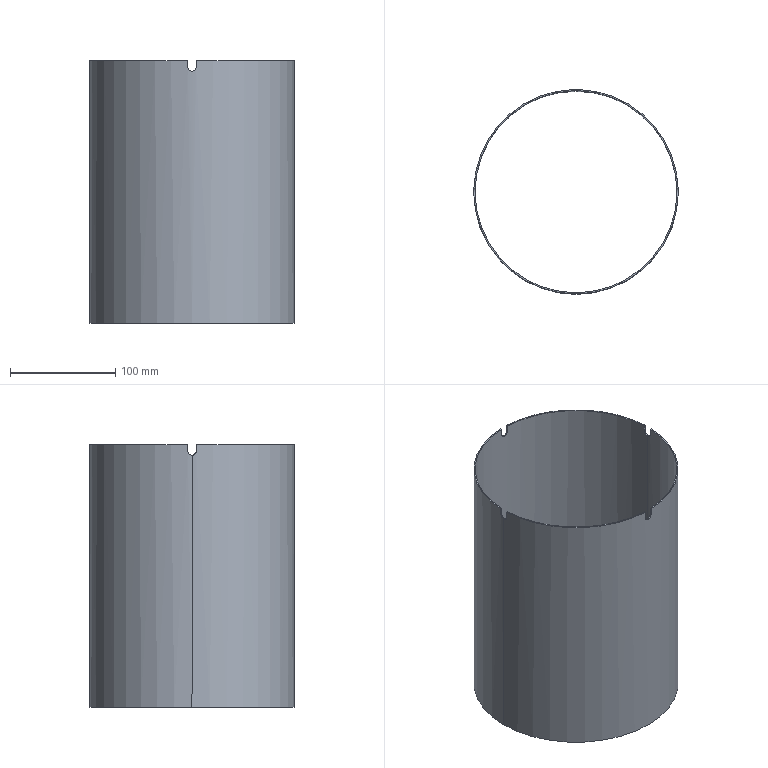Part | SolidWorks | features BaseBody 1 | 1 solid | 23 faces | box 194.5 x 194.5 x 250 mm | volume 181834 mm3 | plane 13 | spline 6 | cylinder 4 | commonest cylinder face diameters 192.1 x2 194.5 x2
STEP:
#1=CARTESIAN_POINT('',(97.25,0.,0.));
#2=VERTEX_POINT('',#1);
#3=CARTESIAN_POINT('',(-97.25,0.,0.));
#4=VERTEX_POINT('',#3);
#5=CARTESIAN_POINT('',(0.,0.,0.));
#6=DIRECTION('',(0.,0.,1.));
#7=DIRECTION('',(1.,0.,0.));
#8=AXIS2_PLACEMENT_3D('',#5,#6,#7);
#9=CIRCLE('',#8,97.25);
#10=EDGE_CURVE('',#2,#4,#9,.T.);
#11=ORIENTED_EDGE('',*,*,#10,.T.);
#12=CARTESIAN_POINT('',(-97.25,0.,240.));
#13=VERTEX_POINT('',#12);
#14=CARTESIAN_POINT('',(-97.25,0.,0.));
#15=DIRECTION('',(0.,0.,1.));
#16=VECTOR('',#15,1000.);
#17=LINE('',#14,#16);
#18=EDGE_CURVE('',#4,#13,#17,.T.);
#19=ORIENTED_EDGE('',*,*,#18,.T.);
#20=CARTESIAN_POINT('',(-97.168,4.,244.));
#21=VERTEX_POINT('',#20);
#22=CARTESIAN_POINT('',(-97.25,0.,240.));
#23=CARTESIAN_POINT('',(-97.25,0.2637,240.002));
#24=CARTESIAN_POINT('',(-97.249,0.5235,240.026));
#25=CARTESIAN_POINT('',(-97.245,1.034,240.127));
#26=CARTESIAN_POINT('',(-97.242,1.287,240.204));
#27=CARTESIAN_POINT('',(-97.234,1.772,240.406));
#28=CARTESIAN_POINT('',(-97.23,2.001,240.528));
#29=CARTESIAN_POINT('',(-97.22,2.437,240.817));
#30=CARTESIAN_POINT('',(-97.214,2.643,240.985));
#31=CARTESIAN_POINT('',(-97.204,3.012,241.354));
#32=CARTESIAN_POINT('',(-97.198,3.177,241.555));
#33=CARTESIAN_POINT('',(-97.188,3.468,241.991));
#34=CARTESIAN_POINT('',(-97.184,3.593,242.225));
#35=CARTESIAN_POINT('',(-97.176,3.794,242.706));
#36=CARTESIAN_POINT('',(-97.173,3.871,242.956));
#37=CARTESIAN_POINT('',(-97.169,3.974,243.474));
#38=CARTESIAN_POINT('',(-97.168,3.999,243.736));
#39=CARTESIAN_POINT('',(-97.168,4.,244.));
#40=B_SPLINE_CURVE_WITH_KNOTS('',3,(#22,#23,#24,#25,#26,#27,#28,#29,#30,#31,#32,#33,#34,#35,#36,#37,#38,#39),.UNSPECIFIED.,.F.,.F.,(4,2,2,2,2,2,2,2,4),(0.,0.0007803,0.001561,0.002341,0.003121,0.003902,0.004682,0.005462,0.006243),.UNSPECIFIED.);
#41=EDGE_CURVE('',#13,#21,#40,.T.);
#42=ORIENTED_EDGE('',*,*,#41,.T.);
#43=CARTESIAN_POINT('',(-97.168,4.,250.));
#44=VERTEX_POINT('',#43);
#45=CARTESIAN_POINT('',(-97.168,4.,0.));
#46=DIRECTION('',(0.,0.,1.));
#47=VECTOR('',#46,1000.);
#48=LINE('',#45,#47);
#49=EDGE_CURVE('',#21,#44,#48,.T.);
#50=ORIENTED_EDGE('',*,*,#49,.T.);
#51=CARTESIAN_POINT('',(-4.,97.168,250.));
#52=VERTEX_POINT('',#51);
#53=CARTESIAN_POINT('',(0.,0.,250.));
#54=DIRECTION('',(0.,0.,-1.));
#55=DIRECTION('',(1.,0.,0.));
#56=AXIS2_PLACEMENT_3D('',#53,#54,#55);
#57=CIRCLE('',#56,97.25);
#58=EDGE_CURVE('',#44,#52,#57,.T.);
#59=ORIENTED_EDGE('',*,*,#58,.T.);
#60=CARTESIAN_POINT('',(-4.,97.168,244.));
#61=VERTEX_POINT('',#60);
#62=CARTESIAN_POINT('',(-4.,97.168,0.));
#63=DIRECTION('',(0.,0.,-1.));
#64=VECTOR('',#63,1000.);
#65=LINE('',#62,#64);
#66=EDGE_CURVE('',#52,#61,#65,.T.);
#67=ORIENTED_EDGE('',*,*,#66,.T.);
#68=CARTESIAN_POINT('',(4.,97.168,244.));
#69=VERTEX_POINT('',#68);
#70=CARTESIAN_POINT('',(-4.,97.168,244.));
#71=CARTESIAN_POINT('',(-3.999,97.168,243.736));
#72=CARTESIAN_POINT('',(-3.974,97.169,243.476));
#73=CARTESIAN_POINT('',(-3.873,97.173,242.965));
#74=CARTESIAN_POINT('',(-3.796,97.176,242.712));
#75=CARTESIAN_POINT('',(-3.594,97.184,242.228));
#76=CARTESIAN_POINT('',(-3.472,97.188,241.998));
#77=CARTESIAN_POINT('',(-3.183,97.198,241.563));
#78=CARTESIAN_POINT('',(-3.014,97.203,241.356));
#79=CARTESIAN_POINT('',(-2.645,97.214,240.987));
#80=CARTESIAN_POINT('',(-2.443,97.22,240.822));
#81=CARTESIAN_POINT('',(-2.007,97.23,240.531));
#82=CARTESIAN_POINT('',(-1.773,97.234,240.406));
#83=CARTESIAN_POINT('',(-1.292,97.242,240.206));
#84=CARTESIAN_POINT('',(-1.041,97.245,240.129));
#85=CARTESIAN_POINT('',(-0.5238,97.249,240.025));
#86=CARTESIAN_POINT('',(-0.2642,97.25,240.));
#87=CARTESIAN_POINT('',(0.2574,97.25,240.));
#88=CARTESIAN_POINT('',(0.5221,97.249,240.026));
#89=CARTESIAN_POINT('',(1.036,97.245,240.128));
#90=CARTESIAN_POINT('',(1.285,97.242,240.203));
#91=CARTESIAN_POINT('',(1.769,97.234,240.403));
#92=CARTESIAN_POINT('',(2.004,97.23,240.528));
#93=CARTESIAN_POINT('',(2.438,97.22,240.818));
#94=CARTESIAN_POINT('',(2.64,97.214,240.983));
#95=CARTESIAN_POINT('',(3.013,97.203,241.355));
#96=CARTESIAN_POINT('',(3.179,97.198,241.558));
#97=CARTESIAN_POINT('',(3.468,97.188,241.992));
#98=CARTESIAN_POINT('',(3.593,97.184,242.225));
#99=CARTESIAN_POINT('',(3.795,97.176,242.71));
#100=CARTESIAN_POINT('',(3.872,97.173,242.959));
#101=CARTESIAN_POINT('',(3.973,97.169,243.471));
#102=CARTESIAN_POINT('',(3.999,97.168,243.736));
#103=CARTESIAN_POINT('',(4.,97.168,244.));
#104=B_SPLINE_CURVE_WITH_KNOTS('',3,(#70,#71,#72,#73,#74,#75,#76,#77,#78,#79,#80,#81,#82,#83,#84,#85,#86,#87,#88,#89,#90,#91,#92,#93,#94,#95,#96,#97,#98,#99,#100,#101,#102,#103),.UNSPECIFIED.,.F.,.F.,(4,2,2,2,2,2,2,2,2,2,2,2,2,2,2,2,4),(0.,0.0007808,0.001562,0.002342,0.003123,0.003904,0.004685,0.005466,0.006246,0.007027,0.007808,0.008589,0.009369,0.01015,0.01093,0.01171,0.01249),.UNSPECIFIED.);
#105=EDGE_CURVE('',#61,#69,#104,.T.);
#106=ORIENTED_EDGE('',*,*,#105,.T.);
#107=CARTESIAN_POINT('',(4.,97.168,250.));
#108=VERTEX_POINT('',#107);
#109=CARTESIAN_POINT('',(4.,97.168,0.));
#110=DIRECTION('',(0.,0.,1.));
#111=VECTOR('',#110,1000.);
#112=LINE('',#109,#111);
#113=EDGE_CURVE('',#69,#108,#112,.T.);
#114=ORIENTED_EDGE('',*,*,#113,.T.);
#115=CARTESIAN_POINT('',(97.168,4.,250.));
#116=VERTEX_POINT('',#115);
#117=CARTESIAN_POINT('',(0.,0.,250.));
#118=DIRECTION('',(0.,0.,-1.));
#119=DIRECTION('',(1.,0.,0.));
#120=AXIS2_PLACEMENT_3D('',#117,#118,#119);
#121=CIRCLE('',#120,97.25);
#122=EDGE_CURVE('',#108,#116,#121,.T.);
#123=ORIENTED_EDGE('',*,*,#122,.T.);
#124=CARTESIAN_POINT('',(97.168,4.,244.));
#125=VERTEX_POINT('',#124);
#126=CARTESIAN_POINT('',(97.168,4.,0.));
#127=DIRECTION('',(0.,0.,-1.));
#128=VECTOR('',#127,1000.);
#129=LINE('',#126,#128);
#130=EDGE_CURVE('',#116,#125,#129,.T.);
#131=ORIENTED_EDGE('',*,*,#130,.T.);
#132=CARTESIAN_POINT('',(97.25,0.,240.));
#133=VERTEX_POINT('',#132);
#134=CARTESIAN_POINT('',(97.168,4.,244.));
#135=CARTESIAN_POINT('',(97.168,3.999,243.736));
#136=CARTESIAN_POINT('',(97.169,3.974,243.476));
#137=CARTESIAN_POINT('',(97.173,3.873,242.966));
#138=CARTESIAN_POINT('',(97.176,3.796,242.713));
#139=CARTESIAN_POINT('',(97.184,3.594,242.228));
#140=CARTESIAN_POINT('',(97.188,3.472,241.999));
#141=CARTESIAN_POINT('',(97.198,3.183,241.563));
#142=CARTESIAN_POINT('',(97.203,3.015,241.357));
#143=CARTESIAN_POINT('',(97.214,2.646,240.988));
#144=CARTESIAN_POINT('',(97.22,2.445,240.823));
#145=CARTESIAN_POINT('',(97.23,2.008,240.532));
#146=CARTESIAN_POINT('',(97.234,1.775,240.407));
#147=CARTESIAN_POINT('',(97.242,1.294,240.206));
#148=CARTESIAN_POINT('',(97.245,1.043,240.129));
#149=CARTESIAN_POINT('',(97.249,0.5258,240.026));
#150=CARTESIAN_POINT('',(97.25,0.2641,240.002));
#151=CARTESIAN_POINT('',(97.25,0.,240.));
#152=B_SPLINE_CURVE_WITH_KNOTS('',3,(#134,#135,#136,#137,#138,#139,#140,#141,#142,#143,#144,#145,#146,#147,#148,#149,#150,#151),.UNSPECIFIED.,.F.,.F.,(4,2,2,2,2,2,2,2,4),(0.,0.0007804,0.001561,0.002341,0.003122,0.003902,0.004683,0.005463,0.006243),.UNSPECIFIED.);
#153=EDGE_CURVE('',#125,#133,#152,.T.);
#154=ORIENTED_EDGE('',*,*,#153,.T.);
#155=CARTESIAN_POINT('',(97.25,0.,0.));
#156=DIRECTION('',(0.,0.,1.));
#157=VECTOR('',#156,1000.);
#158=LINE('',#155,#157);
#159=EDGE_CURVE('',#2,#133,#158,.T.);
#160=ORIENTED_EDGE('',*,*,#159,.F.);
#161=EDGE_LOOP('',(#11,#19,#42,#50,#59,#67,#106,#114,#123,#131,#154,#160));
#162=FACE_OUTER_BOUND('',#161,.T.);
#163=CARTESIAN_POINT('',(0.,0.,0.));
#164=DIRECTION('',(0.,0.,1.));
#165=DIRECTION('',(1.,0.,0.));
#166=AXIS2_PLACEMENT_3D('',#163,#164,#165);
#167=CYLINDRICAL_SURFACE('',#166,97.25);
#168=ADVANCED_FACE('',(#162),#167,.T.);
#169=CARTESIAN_POINT('',(-96.05,0.,0.));
#170=VERTEX_POINT('',#169);
#171=CARTESIAN_POINT('',(96.05,0.,0.));
#172=VERTEX_POINT('',#171);
#173=CARTESIAN_POINT('',(0.,0.,0.));
#174=DIRECTION('',(0.,0.,1.));
#175=DIRECTION('',(1.,0.,0.));
#176=AXIS2_PLACEMENT_3D('',#173,#174,#175);
#177=CIRCLE('',#176,96.05);
#178=EDGE_CURVE('',#170,#172,#177,.T.);
#179=ORIENTED_EDGE('',*,*,#178,.F.);
#180=CARTESIAN_POINT('',(-96.05,0.,240.));
#181=VERTEX_POINT('',#180);
#182=CARTESIAN_POINT('',(-96.05,0.,0.));
#183=DIRECTION('',(0.,0.,1.));
#184=VECTOR('',#183,1000.);
#185=LINE('',#182,#184);
#186=EDGE_CURVE('',#170,#181,#185,.T.);
#187=ORIENTED_EDGE('',*,*,#186,.T.);
#188=CARTESIAN_POINT('',(-95.969,-3.951,244.));
#189=VERTEX_POINT('',#188);
#190=CARTESIAN_POINT('',(-96.05,0.,240.));
#191=CARTESIAN_POINT('',(-96.05,-0.2623,240.001));
#192=CARTESIAN_POINT('',(-96.049,-0.5205,240.026));
#193=CARTESIAN_POINT('',(-96.045,-1.028,240.129));
#194=CARTESIAN_POINT('',(-96.042,-1.28,240.207));
#195=CARTESIAN_POINT('',(-96.034,-1.759,240.41));
#196=CARTESIAN_POINT('',(-96.03,-1.987,240.533));
#197=CARTESIAN_POINT('',(-96.02,-2.417,240.824));
#198=CARTESIAN_POINT('',(-96.014,-2.62,240.994));
#199=CARTESIAN_POINT('',(-96.004,-2.982,241.364));
#200=CARTESIAN_POINT('',(-95.999,-3.145,241.566));
#201=CARTESIAN_POINT('',(-95.989,-3.433,242.003));
#202=CARTESIAN_POINT('',(-95.984,-3.554,242.235));
#203=CARTESIAN_POINT('',(-95.977,-3.749,242.714));
#204=CARTESIAN_POINT('',(-95.974,-3.825,242.965));
#205=CARTESIAN_POINT('',(-95.97,-3.926,243.478));
#206=CARTESIAN_POINT('',(-95.969,-3.95,243.738));
#207=CARTESIAN_POINT('',(-95.969,-3.951,244.));
#208=B_SPLINE_CURVE_WITH_KNOTS('',3,(#190,#191,#192,#193,#194,#195,#196,#197,#198,#199,#200,#201,#202,#203,#204,#205,#206,#207),.UNSPECIFIED.,.F.,.F.,(4,2,2,2,2,2,2,2,4),(0.,0.000776,0.001552,0.002328,0.003104,0.00388,0.004656,0.005432,0.006208),.UNSPECIFIED.);
#209=EDGE_CURVE('',#181,#189,#208,.T.);
#210=ORIENTED_EDGE('',*,*,#209,.T.);
#211=CARTESIAN_POINT('',(-95.969,-3.951,250.));
#212=VERTEX_POINT('',#211);
#213=CARTESIAN_POINT('',(-95.969,-3.951,247.));
#214=DIRECTION('',(0.,0.,1.));
#215=VECTOR('',#214,1000.);
#216=LINE('',#213,#215);
#217=EDGE_CURVE('',#189,#212,#216,.T.);
#218=ORIENTED_EDGE('',*,*,#217,.T.);
#219=CARTESIAN_POINT('',(-3.951,-95.969,250.));
#220=VERTEX_POINT('',#219);
#221=CARTESIAN_POINT('',(0.,0.,250.));
#222=DIRECTION('',(0.,0.,1.));
#223=DIRECTION('',(1.,0.,0.));
#224=AXIS2_PLACEMENT_3D('',#221,#222,#223);
#225=CIRCLE('',#224,96.05);
#226=EDGE_CURVE('',#212,#220,#225,.T.);
#227=ORIENTED_EDGE('',*,*,#226,.T.);
#228=CARTESIAN_POINT('',(-3.951,-95.969,244.));
#229=VERTEX_POINT('',#228);
#230=CARTESIAN_POINT('',(-3.951,-95.969,247.));
#231=DIRECTION('',(0.,0.,1.));
#232=VECTOR('',#231,1000.);
#233=LINE('',#230,#232);
#234=EDGE_CURVE('',#229,#220,#233,.T.);
#235=ORIENTED_EDGE('',*,*,#234,.F.);
#236=CARTESIAN_POINT('',(3.951,-95.969,244.));
#237=VERTEX_POINT('',#236);
#238=CARTESIAN_POINT('',(-3.951,-95.969,244.));
#239=CARTESIAN_POINT('',(-3.949,-95.969,243.738));
#240=CARTESIAN_POINT('',(-3.925,-95.97,243.479));
#241=CARTESIAN_POINT('',(-3.827,-95.974,242.972));
#242=CARTESIAN_POINT('',(-3.751,-95.977,242.72));
#243=CARTESIAN_POINT('',(-3.554,-95.984,242.237));
#244=CARTESIAN_POINT('',(-3.434,-95.989,242.007));
#245=CARTESIAN_POINT('',(-3.151,-95.998,241.573));
#246=CARTESIAN_POINT('',(-2.985,-96.004,241.366));
#247=CARTESIAN_POINT('',(-2.622,-96.014,240.996));
#248=CARTESIAN_POINT('',(-2.423,-96.02,240.83));
#249=CARTESIAN_POINT('',(-1.993,-96.03,240.537));
#250=CARTESIAN_POINT('',(-1.761,-96.034,240.41));
#251=CARTESIAN_POINT('',(-1.284,-96.042,240.208));
#252=CARTESIAN_POINT('',(-1.036,-96.045,240.131));
#253=CARTESIAN_POINT('',(-0.5214,-96.049,240.026));
#254=CARTESIAN_POINT('',(-0.2631,-96.05,240.));
#255=CARTESIAN_POINT('',(0.255,-96.05,240.));
#256=CARTESIAN_POINT('',(0.5178,-96.049,240.026));
#257=CARTESIAN_POINT('',(1.029,-96.045,240.129));
#258=CARTESIAN_POINT('',(1.276,-96.042,240.205));
#259=CARTESIAN_POINT('',(1.756,-96.034,240.407));
#260=CARTESIAN_POINT('',(1.988,-96.03,240.534));
#261=CARTESIAN_POINT('',(2.417,-96.02,240.825));
#262=CARTESIAN_POINT('',(2.616,-96.015,240.991));
#263=CARTESIAN_POINT('',(2.984,-96.004,241.365));
#264=CARTESIAN_POINT('',(3.147,-95.999,241.568));
#265=CARTESIAN_POINT('',(3.431,-95.989,242.001));
#266=CARTESIAN_POINT('',(3.553,-95.984,242.234));
#267=CARTESIAN_POINT('',(3.751,-95.977,242.717));
#268=CARTESIAN_POINT('',(3.825,-95.974,242.965));
#269=CARTESIAN_POINT('',(3.925,-95.97,243.475));
#270=CARTESIAN_POINT('',(3.949,-95.969,243.737));
#271=CARTESIAN_POINT('',(3.951,-95.969,244.));
#272=B_SPLINE_CURVE_WITH_KNOTS('',3,(#238,#239,#240,#241,#242,#243,#244,#245,#246,#247,#248,#249,#250,#251,#252,#253,#254,#255,#256,#257,#258,#259,#260,#261,#262,#263,#264,#265,#266,#267,#268,#269,#270,#271),.UNSPECIFIED.,.F.,.F.,(4,2,2,2,2,2,2,2,2,2,2,2,2,2,2,2,4),(0.,0.0007758,0.001552,0.002328,0.003103,0.003879,0.004655,0.005431,0.006207,0.006983,0.007758,0.008534,0.00931,0.01009,0.01086,0.01164,0.01241),.UNSPECIFIED.);
#273=EDGE_CURVE('',#229,#237,#272,.T.);
#274=ORIENTED_EDGE('',*,*,#273,.T.);
#275=CARTESIAN_POINT('',(3.951,-95.969,250.));
#276=VERTEX_POINT('',#275);
#277=CARTESIAN_POINT('',(3.951,-95.969,247.));
#278=DIRECTION('',(0.,0.,1.));
#279=VECTOR('',#278,1000.);
#280=LINE('',#277,#279);
#281=EDGE_CURVE('',#237,#276,#280,.T.);
#282=ORIENTED_EDGE('',*,*,#281,.T.);
#283=CARTESIAN_POINT('',(95.969,-3.951,250.));
#284=VERTEX_POINT('',#283);
#285=CARTESIAN_POINT('',(0.,0.,250.));
#286=DIRECTION('',(0.,0.,1.));
#287=DIRECTION('',(1.,0.,0.));
#288=AXIS2_PLACEMENT_3D('',#285,#286,#287);
#289=CIRCLE('',#288,96.05);
#290=EDGE_CURVE('',#276,#284,#289,.T.);
#291=ORIENTED_EDGE('',*,*,#290,.T.);
#292=CARTESIAN_POINT('',(95.969,-3.951,244.));
#293=VERTEX_POINT('',#292);
#294=CARTESIAN_POINT('',(95.969,-3.951,247.));
#295=DIRECTION('',(0.,0.,1.));
#296=VECTOR('',#295,1000.);
#297=LINE('',#294,#296);
#298=EDGE_CURVE('',#293,#284,#297,.T.);
#299=ORIENTED_EDGE('',*,*,#298,.F.);
#300=CARTESIAN_POINT('',(96.05,0.,240.));
#301=VERTEX_POINT('',#300);
#302=CARTESIAN_POINT('',(95.969,-3.951,244.));
#303=CARTESIAN_POINT('',(95.969,-3.95,243.738));
#304=CARTESIAN_POINT('',(95.97,-3.926,243.479));
#305=CARTESIAN_POINT('',(95.974,-3.826,242.972));
#306=CARTESIAN_POINT('',(95.977,-3.751,242.719));
#307=CARTESIAN_POINT('',(95.984,-3.555,242.236));
#308=CARTESIAN_POINT('',(95.989,-3.435,242.007));
#309=CARTESIAN_POINT('',(95.998,-3.151,241.574));
#310=CARTESIAN_POINT('',(96.004,-2.985,241.367));
#311=CARTESIAN_POINT('',(96.014,-2.622,240.996));
#312=CARTESIAN_POINT('',(96.02,-2.424,240.83));
#313=CARTESIAN_POINT('',(96.03,-1.994,240.537));
#314=CARTESIAN_POINT('',(96.034,-1.762,240.411));
#315=CARTESIAN_POINT('',(96.042,-1.285,240.209));
#316=CARTESIAN_POINT('',(96.045,-1.037,240.131));
#317=CARTESIAN_POINT('',(96.049,-0.5226,240.026));
#318=CARTESIAN_POINT('',(96.05,-0.2626,240.));
#319=CARTESIAN_POINT('',(96.05,0.,240.));
#320=B_SPLINE_CURVE_WITH_KNOTS('',3,(#302,#303,#304,#305,#306,#307,#308,#309,#310,#311,#312,#313,#314,#315,#316,#317,#318,#319),.UNSPECIFIED.,.F.,.F.,(4,2,2,2,2,2,2,2,4),(0.,0.000776,0.001552,0.002328,0.003104,0.00388,0.004656,0.005432,0.006208),.UNSPECIFIED.);
#321=EDGE_CURVE('',#293,#301,#320,.T.);
#322=ORIENTED_EDGE('',*,*,#321,.T.);
#323=CARTESIAN_POINT('',(96.05,0.,0.));
#324=DIRECTION('',(0.,0.,1.));
#325=VECTOR('',#324,1000.);
#326=LINE('',#323,#325);
#327=EDGE_CURVE('',#172,#301,#326,.T.);
#328=ORIENTED_EDGE('',*,*,#327,.F.);
#329=EDGE_LOOP('',(#179,#187,#210,#218,#227,#235,#274,#282,#291,#299,#322,#328));
#330=FACE_OUTER_BOUND('',#329,.T.);
#331=CARTESIAN_POINT('',(0.,0.,0.));
#332=DIRECTION('',(0.,0.,1.));
#333=DIRECTION('',(1.,0.,0.));
#334=AXIS2_PLACEMENT_3D('',#331,#332,#333);
#335=CYLINDRICAL_SURFACE('',#334,96.05);
#336=ADVANCED_FACE('',(#330),#335,.F.);
#337=ORIENTED_EDGE('',*,*,#18,.F.);
#338=CARTESIAN_POINT('',(0.,0.,0.));
#339=DIRECTION('',(0.,0.,1.));
#340=DIRECTION('',(1.,0.,0.));
#341=AXIS2_PLACEMENT_3D('',#338,#339,#340);
#342=CIRCLE('',#341,97.25);
#343=EDGE_CURVE('',#4,#2,#342,.T.);
#344=ORIENTED_EDGE('',*,*,#343,.T.);
#345=ORIENTED_EDGE('',*,*,#159,.T.);
#346=CARTESIAN_POINT('',(97.168,-4.,244.));
#347=VERTEX_POINT('',#346);
#348=CARTESIAN_POINT('',(97.25,0.,240.));
#349=CARTESIAN_POINT('',(97.25,-0.2639,240.));
#350=CARTESIAN_POINT('',(97.249,-0.5237,240.025));
#351=CARTESIAN_POINT('',(97.245,-1.034,240.127));
#352=CARTESIAN_POINT('',(97.242,-1.288,240.205));
#353=CARTESIAN_POINT('',(97.234,-1.772,240.405));
#354=CARTESIAN_POINT('',(97.23,-2.002,240.527));
#355=CARTESIAN_POINT('',(97.22,-2.437,240.817));
#356=CARTESIAN_POINT('',(97.214,-2.643,240.986));
#357=CARTESIAN_POINT('',(97.204,-3.012,241.355));
#358=CARTESIAN_POINT('',(97.198,-3.177,241.556));
#359=CARTESIAN_POINT('',(97.188,-3.47,241.993));
#360=CARTESIAN_POINT('',(97.184,-3.594,242.226));
#361=CARTESIAN_POINT('',(97.176,-3.794,242.706));
#362=CARTESIAN_POINT('',(97.173,-3.871,242.958));
#363=CARTESIAN_POINT('',(97.169,-3.974,243.475));
#364=CARTESIAN_POINT('',(97.168,-3.999,243.736));
#365=CARTESIAN_POINT('',(97.168,-4.,244.));
#366=B_SPLINE_CURVE_WITH_KNOTS('',3,(#348,#349,#350,#351,#352,#353,#354,#355,#356,#357,#358,#359,#360,#361,#362,#363,#364,#365),.UNSPECIFIED.,.F.,.F.,(4,2,2,2,2,2,2,2,4),(0.,0.0007808,0.001562,0.002342,0.003123,0.003904,0.004685,0.005466,0.006247),.UNSPECIFIED.);
#367=EDGE_CURVE('',#133,#347,#366,.T.);
#368=ORIENTED_EDGE('',*,*,#367,.T.);
#369=CARTESIAN_POINT('',(97.168,-4.,250.));
#370=VERTEX_POINT('',#369);
#371=CARTESIAN_POINT('',(97.168,-4.,0.));
#372=DIRECTION('',(0.,0.,1.));
#373=VECTOR('',#372,1000.);
#374=LINE('',#371,#373);
#375=EDGE_CURVE('',#347,#370,#374,.T.);
#376=ORIENTED_EDGE('',*,*,#375,.T.);
#377=CARTESIAN_POINT('',(4.,-97.168,250.));
#378=VERTEX_POINT('',#377);
#379=CARTESIAN_POINT('',(0.,0.,250.));
#380=DIRECTION('',(0.,0.,-1.));
#381=DIRECTION('',(1.,0.,0.));
#382=AXIS2_PLACEMENT_3D('',#379,#380,#381);
#383=CIRCLE('',#382,97.25);
#384=EDGE_CURVE('',#370,#378,#383,.T.);
#385=ORIENTED_EDGE('',*,*,#384,.T.);
#386=CARTESIAN_POINT('',(4.,-97.168,244.));
#387=VERTEX_POINT('',#386);
#388=CARTESIAN_POINT('',(4.,-97.168,0.));
#389=DIRECTION('',(0.,0.,-1.));
#390=VECTOR('',#389,1000.);
#391=LINE('',#388,#390);
#392=EDGE_CURVE('',#378,#387,#391,.T.);
#393=ORIENTED_EDGE('',*,*,#392,.T.);
#394=CARTESIAN_POINT('',(-4.,-97.168,244.));
#395=VERTEX_POINT('',#394);
#396=CARTESIAN_POINT('',(4.,-97.168,244.));
#397=CARTESIAN_POINT('',(3.999,-97.168,243.736));
#398=CARTESIAN_POINT('',(3.974,-97.169,243.476));
#399=CARTESIAN_POINT('',(3.873,-97.173,242.965));
#400=CARTESIAN_POINT('',(3.796,-97.176,242.712));
#401=CARTESIAN_POINT('',(3.594,-97.184,242.228));
#402=CARTESIAN_POINT('',(3.472,-97.188,241.998));
#403=CARTESIAN_POINT('',(3.183,-97.198,241.563));
#404=CARTESIAN_POINT('',(3.014,-97.203,241.357));
#405=CARTESIAN_POINT('',(2.645,-97.214,240.988));
#406=CARTESIAN_POINT('',(2.443,-97.22,240.822));
#407=CARTESIAN_POINT('',(2.007,-97.23,240.53));
#408=CARTESIAN_POINT('',(1.774,-97.234,240.405));
#409=CARTESIAN_POINT('',(1.292,-97.242,240.205));
#410=CARTESIAN_POINT('',(1.041,-97.245,240.129));
#411=CARTESIAN_POINT('',(0.5239,-97.249,240.026));
#412=CARTESIAN_POINT('',(0.2642,-97.25,240.));
#413=CARTESIAN_POINT('',(-0.2575,-97.25,240.));
#414=CARTESIAN_POINT('',(-0.5223,-97.249,240.025));
#415=CARTESIAN_POINT('',(-1.036,-97.245,240.127));
#416=CARTESIAN_POINT('',(-1.285,-97.242,240.203));
#417=CARTESIAN_POINT('',(-1.769,-97.234,240.404));
#418=CARTESIAN_POINT('',(-2.003,-97.23,240.529));
#419=CARTESIAN_POINT('',(-2.438,-97.22,240.818));
#420=CARTESIAN_POINT('',(-2.64,-97.214,240.983));
#421=CARTESIAN_POINT('',(-3.013,-97.203,241.355));
#422=CARTESIAN_POINT('',(-3.179,-97.198,241.558));
#423=CARTESIAN_POINT('',(-3.468,-97.188,241.992));
#424=CARTESIAN_POINT('',(-3.593,-97.184,242.225));
#425=CARTESIAN_POINT('',(-3.795,-97.176,242.71));
#426=CARTESIAN_POINT('',(-3.872,-97.173,242.959));
#427=CARTESIAN_POINT('',(-3.973,-97.169,243.471));
#428=CARTESIAN_POINT('',(-3.999,-97.168,243.736));
#429=CARTESIAN_POINT('',(-4.,-97.168,244.));
#430=B_SPLINE_CURVE_WITH_KNOTS('',3,(#396,#397,#398,#399,#400,#401,#402,#403,#404,#405,#406,#407,#408,#409,#410,#411,#412,#413,#414,#415,#416,#417,#418,#419,#420,#421,#422,#423,#424,#425,#426,#427,#428,#429),.UNSPECIFIED.,.F.,.F.,(4,2,2,2,2,2,2,2,2,2,2,2,2,2,2,2,4),(0.,0.0007808,0.001562,0.002342,0.003123,0.003904,0.004685,0.005466,0.006246,0.007027,0.007808,0.008589,0.009369,0.01015,0.01093,0.01171,0.01249),.UNSPECIFIED.);
#431=EDGE_CURVE('',#387,#395,#430,.T.);
#432=ORIENTED_EDGE('',*,*,#431,.T.);
#433=CARTESIAN_POINT('',(-4.,-97.168,250.));
#434=VERTEX_POINT('',#433);
#435=CARTESIAN_POINT('',(-4.,-97.168,0.));
#436=DIRECTION('',(0.,0.,1.));
#437=VECTOR('',#436,1000.);
#438=LINE('',#435,#437);
#439=EDGE_CURVE('',#395,#434,#438,.T.);
#440=ORIENTED_EDGE('',*,*,#439,.T.);
#441=CARTESIAN_POINT('',(-97.168,-4.,250.));
#442=VERTEX_POINT('',#441);
#443=CARTESIAN_POINT('',(0.,0.,250.));
#444=DIRECTION('',(0.,0.,-1.));
#445=DIRECTION('',(1.,0.,0.));
#446=AXIS2_PLACEMENT_3D('',#443,#444,#445);
#447=CIRCLE('',#446,97.25);
#448=EDGE_CURVE('',#434,#442,#447,.T.);
#449=ORIENTED_EDGE('',*,*,#448,.T.);
#450=CARTESIAN_POINT('',(-97.168,-4.,244.));
#451=VERTEX_POINT('',#450);
#452=CARTESIAN_POINT('',(-97.168,-4.,0.));
#453=DIRECTION('',(0.,0.,-1.));
#454=VECTOR('',#453,1000.);
#455=LINE('',#452,#454);
#456=EDGE_CURVE('',#442,#451,#455,.T.);
#457=ORIENTED_EDGE('',*,*,#456,.T.);
#458=CARTESIAN_POINT('',(-97.168,-4.,244.));
#459=CARTESIAN_POINT('',(-97.168,-3.999,243.736));
#460=CARTESIAN_POINT('',(-97.169,-3.974,243.476));
#461=CARTESIAN_POINT('',(-97.173,-3.873,242.965));
#462=CARTESIAN_POINT('',(-97.176,-3.796,242.712));
#463=CARTESIAN_POINT('',(-97.184,-3.595,242.228));
#464=CARTESIAN_POINT('',(-97.188,-3.473,241.998));
#465=CARTESIAN_POINT('',(-97.198,-3.183,241.564));
#466=CARTESIAN_POINT('',(-97.203,-3.014,241.358));
#467=CARTESIAN_POINT('',(-97.214,-2.646,240.988));
#468=CARTESIAN_POINT('',(-97.22,-2.445,240.822));
#469=CARTESIAN_POINT('',(-97.23,-2.008,240.531));
#470=CARTESIAN_POINT('',(-97.234,-1.775,240.407));
#471=CARTESIAN_POINT('',(-97.242,-1.294,240.207));
#472=CARTESIAN_POINT('',(-97.245,-1.043,240.129));
#473=CARTESIAN_POINT('',(-97.249,-0.5256,240.025));
#474=CARTESIAN_POINT('',(-97.25,-0.2641,240.001));
#475=CARTESIAN_POINT('',(-97.25,0.,240.));
#476=B_SPLINE_CURVE_WITH_KNOTS('',3,(#458,#459,#460,#461,#462,#463,#464,#465,#466,#467,#468,#469,#470,#471,#472,#473,#474,#475),.UNSPECIFIED.,.F.,.F.,(4,2,2,2,2,2,2,2,4),(0.,0.0007809,0.001562,0.002343,0.003123,0.003904,0.004685,0.005466,0.006247),.UNSPECIFIED.);
#477=EDGE_CURVE('',#451,#13,#476,.T.);
#478=ORIENTED_EDGE('',*,*,#477,.T.);
#479=EDGE_LOOP('',(#337,#344,#345,#368,#376,#385,#393,#432,#440,#449,#457,#478));
#480=FACE_OUTER_BOUND('',#479,.T.);
#481=CARTESIAN_POINT('',(0.,0.,0.));
#482=DIRECTION('',(0.,0.,1.));
#483=DIRECTION('',(1.,0.,0.));
#484=AXIS2_PLACEMENT_3D('',#481,#482,#483);
#485=CYLINDRICAL_SURFACE('',#484,97.25);
#486=ADVANCED_FACE('',(#480),#485,.T.);
#487=CARTESIAN_POINT('',(3.951,95.969,250.));
#488=VERTEX_POINT('',#487);
#489=CARTESIAN_POINT('',(3.975,96.568,250.));
#490=DIRECTION('',(0.04113,0.9992,0.));
#491=VECTOR('',#490,1000.);
#492=LINE('',#489,#491);
#493=EDGE_CURVE('',#488,#108,#492,.T.);
#494=ORIENTED_EDGE('',*,*,#493,.T.);
#495=ORIENTED_EDGE('',*,*,#113,.F.);
#496=CARTESIAN_POINT('',(3.951,95.969,244.));
#497=VERTEX_POINT('',#496);
#498=CARTESIAN_POINT('',(3.975,96.568,244.));
#499=DIRECTION('',(-0.04113,-0.9992,0.));
#500=VECTOR('',#499,1000.);
#501=LINE('',#498,#500);
#502=EDGE_CURVE('',#69,#497,#501,.T.);
#503=ORIENTED_EDGE('',*,*,#502,.T.);
#504=CARTESIAN_POINT('',(3.951,95.969,247.));
#505=DIRECTION('',(0.,0.,1.));
#506=VECTOR('',#505,1000.);
#507=LINE('',#504,#506);
#508=EDGE_CURVE('',#497,#488,#507,.T.);
#509=ORIENTED_EDGE('',*,*,#508,.T.);
#510=EDGE_LOOP('',(#494,#495,#503,#509));
#511=FACE_OUTER_BOUND('',#510,.T.);
#512=CARTESIAN_POINT('',(3.975,96.568,247.));
#513=DIRECTION('',(-0.9992,0.04113,0.));
#514=DIRECTION('',(-0.04113,-0.9992,0.));
#515=AXIS2_PLACEMENT_3D('',#512,#513,#514);
#516=PLANE('',#515);
#517=ADVANCED_FACE('',(#511),#516,.T.);
#518=CARTESIAN_POINT('',(-3.951,95.969,244.));
#519=VERTEX_POINT('',#518);
#520=CARTESIAN_POINT('',(3.951,95.969,244.));
#521=CARTESIAN_POINT('',(3.949,95.969,243.738));
#522=CARTESIAN_POINT('',(3.925,95.97,243.479));
#523=CARTESIAN_POINT('',(3.827,95.974,242.972));
#524=CARTESIAN_POINT('',(3.752,95.977,242.72));
#525=CARTESIAN_POINT('',(3.554,95.984,242.237));
#526=CARTESIAN_POINT('',(3.434,95.989,242.007));
#527=CARTESIAN_POINT('',(3.151,95.998,241.573));
#528=CARTESIAN_POINT('',(2.985,96.004,241.367));
#529=CARTESIAN_POINT('',(2.621,96.014,240.996));
#530=CARTESIAN_POINT('',(2.423,96.02,240.83));
#531=CARTESIAN_POINT('',(1.993,96.03,240.536));
#532=CARTESIAN_POINT('',(1.761,96.034,240.41));
#533=CARTESIAN_POINT('',(1.284,96.042,240.208));
#534=CARTESIAN_POINT('',(1.036,96.045,240.131));
#535=CARTESIAN_POINT('',(0.5215,96.049,240.027));
#536=CARTESIAN_POINT('',(0.2631,96.05,240.));
#537=CARTESIAN_POINT('',(-0.2551,96.05,240.));
#538=CARTESIAN_POINT('',(-0.518,96.049,240.025));
#539=CARTESIAN_POINT('',(-1.029,96.045,240.129));
#540=CARTESIAN_POINT('',(-1.276,96.042,240.205));
#541=CARTESIAN_POINT('',(-1.755,96.034,240.408));
#542=CARTESIAN_POINT('',(-1.988,96.03,240.534));
#543=CARTESIAN_POINT('',(-2.417,96.02,240.825));
#544=CARTESIAN_POINT('',(-2.616,96.015,240.991));
#545=CARTESIAN_POINT('',(-2.984,96.004,241.364));
#546=CARTESIAN_POINT('',(-3.147,95.999,241.568));
#547=CARTESIAN_POINT('',(-3.431,95.989,242.001));
#548=CARTESIAN_POINT('',(-3.553,95.984,242.234));
#549=CARTESIAN_POINT('',(-3.751,95.977,242.717));
#550=CARTESIAN_POINT('',(-3.825,95.974,242.965));
#551=CARTESIAN_POINT('',(-3.925,95.97,243.475));
#552=CARTESIAN_POINT('',(-3.949,95.969,243.737));
#553=CARTESIAN_POINT('',(-3.951,95.969,244.));
#554=B_SPLINE_CURVE_WITH_KNOTS('',3,(#520,#521,#522,#523,#524,#525,#526,#527,#528,#529,#530,#531,#532,#533,#534,#535,#536,#537,#538,#539,#540,#541,#542,#543,#544,#545,#546,#547,#548,#549,#550,#551,#552,#553),.UNSPECIFIED.,.F.,.F.,(4,2,2,2,2,2,2,2,2,2,2,2,2,2,2,2,4),(0.,0.0007758,0.001552,0.002328,0.003103,0.003879,0.004655,0.005431,0.006207,0.006983,0.007758,0.008534,0.00931,0.01009,0.01086,0.01164,0.01241),.UNSPECIFIED.);
#555=EDGE_CURVE('',#497,#519,#554,.T.);
#556=ORIENTED_EDGE('',*,*,#555,.F.);
#557=ORIENTED_EDGE('',*,*,#502,.F.);
#558=ORIENTED_EDGE('',*,*,#105,.F.);
#559=CARTESIAN_POINT('',(-3.975,96.568,244.));
#560=DIRECTION('',(-0.04113,0.9992,0.));
#561=VECTOR('',#560,1000.);
#562=LINE('',#559,#561);
#563=EDGE_CURVE('',#519,#61,#562,.T.);
#564=ORIENTED_EDGE('',*,*,#563,.F.);
#565=EDGE_LOOP('',(#556,#557,#558,#564));
#566=FACE_OUTER_BOUND('',#565,.T.);
#567=CARTESIAN_POINT('',(-4.014,97.614,244.224));
#568=CARTESIAN_POINT('',(-3.985,96.917,244.224));
#569=CARTESIAN_POINT('',(-3.957,96.22,244.224));
#570=CARTESIAN_POINT('',(-3.928,95.522,244.224));
#571=CARTESIAN_POINT('',(-4.017,97.614,244.148));
#572=CARTESIAN_POINT('',(-3.989,96.917,244.148));
#573=CARTESIAN_POINT('',(-3.96,96.22,244.148));
#574=CARTESIAN_POINT('',(-3.931,95.522,244.148));
#575=CARTESIAN_POINT('',(-4.027,97.614,243.643));
#576=CARTESIAN_POINT('',(-3.998,96.917,243.643));
#577=CARTESIAN_POINT('',(-3.97,96.219,243.643));
#578=CARTESIAN_POINT('',(-3.941,95.522,243.643));
#579=CARTESIAN_POINT('',(-3.89,97.62,242.761));
#580=CARTESIAN_POINT('',(-3.862,96.922,242.761));
#581=CARTESIAN_POINT('',(-3.834,96.225,242.761));
#582=CARTESIAN_POINT('',(-3.806,95.527,242.761));
#583=CARTESIAN_POINT('',(-3.309,97.642,241.614));
#584=CARTESIAN_POINT('',(-3.285,96.944,241.614));
#585=CARTESIAN_POINT('',(-3.261,96.247,241.614));
#586=CARTESIAN_POINT('',(-3.238,95.549,241.614));
#587=CARTESIAN_POINT('',(-2.409,97.669,240.716));
#588=CARTESIAN_POINT('',(-2.392,96.971,240.716));
#589=CARTESIAN_POINT('',(-2.375,96.274,240.716));
#590=CARTESIAN_POINT('',(-2.358,95.576,240.716));
#591=CARTESIAN_POINT('',(-1.264,97.691,240.133));
#592=CARTESIAN_POINT('',(-1.255,96.993,240.133));
#593=CARTESIAN_POINT('',(-1.246,96.295,240.133));
#594=CARTESIAN_POINT('',(-1.236,95.598,240.133));
#595=CARTESIAN_POINT('',(-0.004386,97.7,239.934));
#596=CARTESIAN_POINT('',(-0.004355,97.002,239.934));
#597=CARTESIAN_POINT('',(-0.004323,96.304,239.934));
#598=CARTESIAN_POINT('',(-0.004292,95.606,239.934));
#599=CARTESIAN_POINT('',(1.265,97.691,240.133));
#600=CARTESIAN_POINT('',(1.256,96.993,240.133));
#601=CARTESIAN_POINT('',(1.247,96.295,240.133));
#602=CARTESIAN_POINT('',(1.238,95.598,240.133));
#603=CARTESIAN_POINT('',(2.403,97.669,240.712));
#604=CARTESIAN_POINT('',(2.386,96.971,240.712));
#605=CARTESIAN_POINT('',(2.368,96.274,240.712));
#606=CARTESIAN_POINT('',(2.351,95.576,240.712));
#607=CARTESIAN_POINT('',(3.308,97.642,241.612));
#608=CARTESIAN_POINT('',(3.285,96.944,241.612));
#609=CARTESIAN_POINT('',(3.261,96.247,241.612));
#610=CARTESIAN_POINT('',(3.237,95.549,241.612));
#611=CARTESIAN_POINT('',(3.889,97.62,242.76));
#612=CARTESIAN_POINT('',(3.861,96.922,242.76));
#613=CARTESIAN_POINT('',(3.834,96.225,242.76));
#614=CARTESIAN_POINT('',(3.806,95.527,242.76));
#615=CARTESIAN_POINT('',(4.027,97.614,243.643));
#616=CARTESIAN_POINT('',(3.999,96.917,243.643));
#617=CARTESIAN_POINT('',(3.97,96.219,243.643));
#618=CARTESIAN_POINT('',(3.941,95.522,243.643));
#619=CARTESIAN_POINT('',(4.017,97.614,244.151));
#620=CARTESIAN_POINT('',(3.989,96.917,244.151));
#621=CARTESIAN_POINT('',(3.96,96.22,244.151));
#622=CARTESIAN_POINT('',(3.931,95.522,244.151));
#623=CARTESIAN_POINT('',(4.014,97.614,244.228));
#624=CARTESIAN_POINT('',(3.985,96.917,244.228));
#625=CARTESIAN_POINT('',(3.956,96.22,244.228));
#626=CARTESIAN_POINT('',(3.928,95.522,244.228));
#627=B_SPLINE_SURFACE_WITH_KNOTS('',3,3,((#567,#568,#569,#570),(#571,#572,#573,#574),(#575,#576,#577,#578),(#579,#580,#581,#582),(#583,#584,#585,#586),(#587,#588,#589,#590),(#591,#592,#593,#594),(#595,#596,#597,#598),(#599,#600,#601,#602),(#603,#604,#605,#606),(#607,#608,#609,#610),(#611,#612,#613,#614),(#615,#616,#617,#618),(#619,#620,#621,#622),(#623,#624,#625,#626)),.UNSPECIFIED.,.F.,.F.,.F.,(4,1,1,1,1,1,1,1,1,1,1,1,4),(4,4),(-0.01728,0.,0.1,0.2,0.3,0.4,0.5,0.6,0.7,0.8,0.9,1.,1.018),(-0.3725,1.372),.UNSPECIFIED.);
#628=ADVANCED_FACE('',(#566),#627,.F.);
#629=CARTESIAN_POINT('',(-3.951,95.969,250.));
#630=VERTEX_POINT('',#629);
#631=CARTESIAN_POINT('',(-3.951,95.969,247.));
#632=DIRECTION('',(0.,0.,1.));
#633=VECTOR('',#632,1000.);
#634=LINE('',#631,#633);
#635=EDGE_CURVE('',#519,#630,#634,.T.);
#636=ORIENTED_EDGE('',*,*,#635,.F.);
#637=ORIENTED_EDGE('',*,*,#563,.T.);
#638=ORIENTED_EDGE('',*,*,#66,.F.);
#639=CARTESIAN_POINT('',(-3.975,96.568,250.));
#640=DIRECTION('',(-0.04113,0.9992,0.));
#641=VECTOR('',#640,1000.);
#642=LINE('',#639,#641);
#643=EDGE_CURVE('',#630,#52,#642,.T.);
#644=ORIENTED_EDGE('',*,*,#643,.F.);
#645=EDGE_LOOP('',(#636,#637,#638,#644));
#646=FACE_OUTER_BOUND('',#645,.T.);
#647=CARTESIAN_POINT('',(-3.975,96.568,247.));
#648=DIRECTION('',(-0.9992,-0.04113,0.));
#649=DIRECTION('',(0.04113,-0.9992,0.));
#650=AXIS2_PLACEMENT_3D('',#647,#648,#649);
#651=PLANE('',#650);
#652=ADVANCED_FACE('',(#646),#651,.F.);
#653=CARTESIAN_POINT('',(-95.969,3.951,250.));
#654=VERTEX_POINT('',#653);
#655=CARTESIAN_POINT('',(-95.969,3.951,250.));
#656=DIRECTION('',(-0.9992,0.04113,0.));
#657=VECTOR('',#656,1000.);
#658=LINE('',#655,#657);
#659=EDGE_CURVE('',#654,#44,#658,.T.);
#660=ORIENTED_EDGE('',*,*,#659,.F.);
#661=CARTESIAN_POINT('',(0.,0.,250.));
#662=DIRECTION('',(0.,0.,1.));
#663=DIRECTION('',(1.,0.,0.));
#664=AXIS2_PLACEMENT_3D('',#661,#662,#663);
#665=CIRCLE('',#664,96.05);
#666=EDGE_CURVE('',#630,#654,#665,.T.);
#667=ORIENTED_EDGE('',*,*,#666,.F.);
#668=ORIENTED_EDGE('',*,*,#643,.T.);
#669=ORIENTED_EDGE('',*,*,#58,.F.);
#670=EDGE_LOOP('',(#660,#667,#668,#669));
#671=FACE_OUTER_BOUND('',#670,.T.);
#672=CARTESIAN_POINT('',(0.,96.65,250.));
#673=DIRECTION('',(0.,0.,-1.));
#674=DIRECTION('',(-1.,0.,0.));
#675=AXIS2_PLACEMENT_3D('',#672,#673,#674);
#676=PLANE('',#675);
#677=ADVANCED_FACE('',(#671),#676,.F.);
#678=ORIENTED_EDGE('',*,*,#659,.T.);
#679=ORIENTED_EDGE('',*,*,#49,.F.);
#680=CARTESIAN_POINT('',(-95.969,3.951,244.));
#681=VERTEX_POINT('',#680);
#682=CARTESIAN_POINT('',(-96.568,3.975,244.));
#683=DIRECTION('',(0.9992,-0.04113,0.));
#684=VECTOR('',#683,1000.);
#685=LINE('',#682,#684);
#686=EDGE_CURVE('',#21,#681,#685,.T.);
#687=ORIENTED_EDGE('',*,*,#686,.T.);
#688=CARTESIAN_POINT('',(-95.969,3.951,247.));
#689=DIRECTION('',(0.,0.,1.));
#690=VECTOR('',#689,1000.);
#691=LINE('',#688,#690);
#692=EDGE_CURVE('',#681,#654,#691,.T.);
#693=ORIENTED_EDGE('',*,*,#692,.T.);
#694=EDGE_LOOP('',(#678,#679,#687,#693));
#695=FACE_OUTER_BOUND('',#694,.T.);
#696=CARTESIAN_POINT('',(-96.568,3.975,247.));
#697=DIRECTION('',(-0.04113,-0.9992,0.));
#698=DIRECTION('',(0.9992,-0.04113,0.));
#699=AXIS2_PLACEMENT_3D('',#696,#697,#698);
#700=PLANE('',#699);
#701=ADVANCED_FACE('',(#695),#700,.T.);
#702=CARTESIAN_POINT('',(-95.969,3.951,244.));
#703=CARTESIAN_POINT('',(-95.969,3.949,243.738));
#704=CARTESIAN_POINT('',(-95.97,3.925,243.48));
#705=CARTESIAN_POINT('',(-95.974,3.827,242.972));
#706=CARTESIAN_POINT('',(-95.977,3.752,242.72));
#707=CARTESIAN_POINT('',(-95.984,3.554,242.237));
#708=CARTESIAN_POINT('',(-95.989,3.434,242.008));
#709=CARTESIAN_POINT('',(-95.998,3.151,241.573));
#710=CARTESIAN_POINT('',(-96.004,2.986,241.366));
#711=CARTESIAN_POINT('',(-96.014,2.623,240.996));
#712=CARTESIAN_POINT('',(-96.02,2.424,240.83));
#713=CARTESIAN_POINT('',(-96.03,1.994,240.538));
#714=CARTESIAN_POINT('',(-96.034,1.762,240.412));
#715=CARTESIAN_POINT('',(-96.042,1.285,240.209));
#716=CARTESIAN_POINT('',(-96.045,1.038,240.131));
#717=CARTESIAN_POINT('',(-96.049,0.5229,240.027));
#718=CARTESIAN_POINT('',(-96.05,0.2626,240.002));
#719=CARTESIAN_POINT('',(-96.05,0.,240.));
#720=B_SPLINE_CURVE_WITH_KNOTS('',3,(#702,#703,#704,#705,#706,#707,#708,#709,#710,#711,#712,#713,#714,#715,#716,#717,#718,#719),.UNSPECIFIED.,.F.,.F.,(4,2,2,2,2,2,2,2,4),(0.,0.0007756,0.001551,0.002327,0.003102,0.003878,0.004654,0.005429,0.006205),.UNSPECIFIED.);
#721=EDGE_CURVE('',#681,#181,#720,.T.);
#722=ORIENTED_EDGE('',*,*,#721,.F.);
#723=ORIENTED_EDGE('',*,*,#686,.F.);
#724=ORIENTED_EDGE('',*,*,#41,.F.);
#725=CARTESIAN_POINT('',(-96.65,0.,240.));
#726=DIRECTION('',(1.,0.,0.));
#727=VECTOR('',#726,1000.);
#728=LINE('',#725,#727);
#729=EDGE_CURVE('',#13,#181,#728,.T.);
#730=ORIENTED_EDGE('',*,*,#729,.T.);
#731=EDGE_LOOP('',(#722,#723,#724,#730));
#732=FACE_OUTER_BOUND('',#731,.T.);
#733=CARTESIAN_POINT('',(-97.697,-0.2246,240.004));
#734=CARTESIAN_POINT('',(-96.999,-0.223,240.004));
#735=CARTESIAN_POINT('',(-96.301,-0.2214,240.004));
#736=CARTESIAN_POINT('',(-95.603,-0.2198,240.004));
#737=CARTESIAN_POINT('',(-97.697,-0.149,240.001));
#738=CARTESIAN_POINT('',(-96.999,-0.148,240.001));
#739=CARTESIAN_POINT('',(-96.301,-0.1469,240.001));
#740=CARTESIAN_POINT('',(-95.603,-0.1458,240.001));
#741=CARTESIAN_POINT('',(-97.697,0.3655,239.992));
#742=CARTESIAN_POINT('',(-96.999,0.3629,239.992));
#743=CARTESIAN_POINT('',(-96.301,0.3603,239.992));
#744=CARTESIAN_POINT('',(-95.603,0.3577,239.992));
#745=CARTESIAN_POINT('',(-97.691,1.26,240.131));
#746=CARTESIAN_POINT('',(-96.993,1.251,240.131));
#747=CARTESIAN_POINT('',(-96.295,1.242,240.131));
#748=CARTESIAN_POINT('',(-95.598,1.233,240.131));
#749=CARTESIAN_POINT('',(-97.669,2.421,240.724));
#750=CARTESIAN_POINT('',(-96.971,2.404,240.724));
#751=CARTESIAN_POINT('',(-96.273,2.386,240.724));
#752=CARTESIAN_POINT('',(-95.576,2.369,240.724));
#753=CARTESIAN_POINT('',(-97.642,3.311,241.619));
#754=CARTESIAN_POINT('',(-96.944,3.288,241.619));
#755=CARTESIAN_POINT('',(-96.247,3.264,241.619));
#756=CARTESIAN_POINT('',(-95.549,3.24,241.619));
#757=CARTESIAN_POINT('',(-97.62,3.891,242.764));
#758=CARTESIAN_POINT('',(-96.922,3.863,242.764));
#759=CARTESIAN_POINT('',(-96.225,3.835,242.764));
#760=CARTESIAN_POINT('',(-95.527,3.807,242.764));
#761=CARTESIAN_POINT('',(-97.614,4.027,243.645));
#762=CARTESIAN_POINT('',(-96.917,3.999,243.645));
#763=CARTESIAN_POINT('',(-96.219,3.97,243.645));
#764=CARTESIAN_POINT('',(-95.522,3.941,243.645));
#765=CARTESIAN_POINT('',(-97.614,4.017,244.151));
#766=CARTESIAN_POINT('',(-96.917,3.989,244.151));
#767=CARTESIAN_POINT('',(-96.22,3.96,244.151));
#768=CARTESIAN_POINT('',(-95.522,3.931,244.151));
#769=CARTESIAN_POINT('',(-97.614,4.014,244.228));
#770=CARTESIAN_POINT('',(-96.917,3.985,244.228));
#771=CARTESIAN_POINT('',(-96.22,3.956,244.228));
#772=CARTESIAN_POINT('',(-95.522,3.928,244.228));
#773=B_SPLINE_SURFACE_WITH_KNOTS('',3,3,((#733,#734,#735,#736),(#737,#738,#739,#740),(#741,#742,#743,#744),(#745,#746,#747,#748),(#749,#750,#751,#752),(#753,#754,#755,#756),(#757,#758,#759,#760),(#761,#762,#763,#764),(#765,#766,#767,#768),(#769,#770,#771,#772)),.UNSPECIFIED.,.F.,.F.,.F.,(4,1,1,1,1,1,1,4),(4,4),(-0.03404,0.,0.2,0.4,0.6,0.8,1.,1.035),(-0.3725,1.372),.UNSPECIFIED.);
#774=ADVANCED_FACE('',(#732),#773,.F.);
#775=CARTESIAN_POINT('',(0.,0.,0.));
#776=DIRECTION('',(0.,0.,1.));
#777=DIRECTION('',(1.,0.,0.));
#778=AXIS2_PLACEMENT_3D('',#775,#776,#777);
#779=CIRCLE('',#778,96.05);
#780=EDGE_CURVE('',#172,#170,#779,.T.);
#781=ORIENTED_EDGE('',*,*,#780,.T.);
#782=ORIENTED_EDGE('',*,*,#178,.T.);
#783=EDGE_LOOP('',(#781,#782));
#784=FACE_BOUND('',#783,.T.);
#785=ORIENTED_EDGE('',*,*,#10,.F.);
#786=ORIENTED_EDGE('',*,*,#343,.F.);
#787=EDGE_LOOP('',(#785,#786));
#788=FACE_OUTER_BOUND('',#787,.T.);
#789=CARTESIAN_POINT('',(0.,96.65,0.));
#790=DIRECTION('',(0.,0.,-1.));
#791=DIRECTION('',(-1.,0.,0.));
#792=AXIS2_PLACEMENT_3D('',#789,#790,#791);
#793=PLANE('',#792);
#794=ADVANCED_FACE('',(#784,#788),#793,.T.);
#795=CARTESIAN_POINT('',(95.969,3.951,244.));
#796=VERTEX_POINT('',#795);
#797=CARTESIAN_POINT('',(96.05,0.,240.));
#798=CARTESIAN_POINT('',(96.05,0.2621,240.002));
#799=CARTESIAN_POINT('',(96.049,0.5202,240.027));
#800=CARTESIAN_POINT('',(96.045,1.027,240.128));
#801=CARTESIAN_POINT('',(96.042,1.279,240.206));
#802=CARTESIAN_POINT('',(96.034,1.759,240.41));
#803=CARTESIAN_POINT('',(96.03,1.986,240.534));
#804=CARTESIAN_POINT('',(96.02,2.416,240.824));
#805=CARTESIAN_POINT('',(96.014,2.62,240.993));
#806=CARTESIAN_POINT('',(96.004,2.983,241.363));
#807=CARTESIAN_POINT('',(95.999,3.145,241.565));
#808=CARTESIAN_POINT('',(95.989,3.431,242.002));
#809=CARTESIAN_POINT('',(95.984,3.553,242.234));
#810=CARTESIAN_POINT('',(95.977,3.749,242.713));
#811=CARTESIAN_POINT('',(95.974,3.825,242.963));
#812=CARTESIAN_POINT('',(95.97,3.925,243.478));
#813=CARTESIAN_POINT('',(95.969,3.949,243.738));
#814=CARTESIAN_POINT('',(95.969,3.951,244.));
#815=B_SPLINE_CURVE_WITH_KNOTS('',3,(#797,#798,#799,#800,#801,#802,#803,#804,#805,#806,#807,#808,#809,#810,#811,#812,#813,#814),.UNSPECIFIED.,.F.,.F.,(4,2,2,2,2,2,2,2,4),(0.,0.0007755,0.001551,0.002327,0.003102,0.003878,0.004653,0.005429,0.006204),.UNSPECIFIED.);
#816=EDGE_CURVE('',#301,#796,#815,.T.);
#817=ORIENTED_EDGE('',*,*,#816,.F.);
#818=CARTESIAN_POINT('',(96.65,0.,240.));
#819=DIRECTION('',(-1.,0.,0.));
#820=VECTOR('',#819,1000.);
#821=LINE('',#818,#820);
#822=EDGE_CURVE('',#133,#301,#821,.T.);
#823=ORIENTED_EDGE('',*,*,#822,.F.);
#824=ORIENTED_EDGE('',*,*,#153,.F.);
#825=CARTESIAN_POINT('',(96.568,3.975,244.));
#826=DIRECTION('',(0.9992,0.04113,0.));
#827=VECTOR('',#826,1000.);
#828=LINE('',#825,#827);
#829=EDGE_CURVE('',#796,#125,#828,.T.);
#830=ORIENTED_EDGE('',*,*,#829,.F.);
#831=EDGE_LOOP('',(#817,#823,#824,#830));
#832=FACE_OUTER_BOUND('',#831,.T.);
#833=CARTESIAN_POINT('',(97.614,4.014,244.224));
#834=CARTESIAN_POINT('',(96.917,3.985,244.224));
#835=CARTESIAN_POINT('',(96.22,3.957,244.224));
#836=CARTESIAN_POINT('',(95.522,3.928,244.224));
#837=CARTESIAN_POINT('',(97.614,4.017,244.148));
#838=CARTESIAN_POINT('',(96.917,3.989,244.148));
#839=CARTESIAN_POINT('',(96.22,3.96,244.148));
#840=CARTESIAN_POINT('',(95.522,3.931,244.148));
#841=CARTESIAN_POINT('',(97.614,4.027,243.644));
#842=CARTESIAN_POINT('',(96.917,3.998,243.644));
#843=CARTESIAN_POINT('',(96.219,3.97,243.644));
#844=CARTESIAN_POINT('',(95.522,3.941,243.644));
#845=CARTESIAN_POINT('',(97.62,3.891,242.765));
#846=CARTESIAN_POINT('',(96.922,3.863,242.765));
#847=CARTESIAN_POINT('',(96.225,3.835,242.765));
#848=CARTESIAN_POINT('',(95.527,3.807,242.765));
#849=CARTESIAN_POINT('',(97.642,3.312,241.62));
#850=CARTESIAN_POINT('',(96.944,3.288,241.62));
#851=CARTESIAN_POINT('',(96.247,3.265,241.62));
#852=CARTESIAN_POINT('',(95.549,3.241,241.62));
#853=CARTESIAN_POINT('',(97.669,2.422,240.724));
#854=CARTESIAN_POINT('',(96.971,2.405,240.724));
#855=CARTESIAN_POINT('',(96.273,2.387,240.724));
#856=CARTESIAN_POINT('',(95.575,2.37,240.724));
#857=CARTESIAN_POINT('',(97.691,1.262,240.131));
#858=CARTESIAN_POINT('',(96.993,1.253,240.131));
#859=CARTESIAN_POINT('',(96.295,1.244,240.131));
#860=CARTESIAN_POINT('',(95.597,1.235,240.131));
#861=CARTESIAN_POINT('',(97.697,0.3652,239.992));
#862=CARTESIAN_POINT('',(96.999,0.3626,239.992));
#863=CARTESIAN_POINT('',(96.301,0.3599,239.992));
#864=CARTESIAN_POINT('',(95.604,0.3573,239.992));
#865=CARTESIAN_POINT('',(97.697,-0.1518,240.001));
#866=CARTESIAN_POINT('',(96.999,-0.1507,240.001));
#867=CARTESIAN_POINT('',(96.301,-0.1496,240.001));
#868=CARTESIAN_POINT('',(95.603,-0.1485,240.001));
#869=CARTESIAN_POINT('',(97.697,-0.2288,240.004));
#870=CARTESIAN_POINT('',(96.999,-0.2272,240.004));
#871=CARTESIAN_POINT('',(96.301,-0.2255,240.004));
#872=CARTESIAN_POINT('',(95.603,-0.2239,240.004));
#873=B_SPLINE_SURFACE_WITH_KNOTS('',3,3,((#833,#834,#835,#836),(#837,#838,#839,#840),(#841,#842,#843,#844),(#845,#846,#847,#848),(#849,#850,#851,#852),(#853,#854,#855,#856),(#857,#858,#859,#860),(#861,#862,#863,#864),(#865,#866,#867,#868),(#869,#870,#871,#872)),.UNSPECIFIED.,.F.,.F.,.F.,(4,1,1,1,1,1,1,4),(4,4),(-0.03467,0.,0.2,0.4,0.6,0.8,1.,1.035),(-0.3725,1.372),.UNSPECIFIED.);
#874=ADVANCED_FACE('',(#832),#873,.F.);
#875=CARTESIAN_POINT('',(95.969,3.951,250.));
#876=VERTEX_POINT('',#875);
#877=CARTESIAN_POINT('',(95.969,3.951,247.));
#878=DIRECTION('',(0.,0.,1.));
#879=VECTOR('',#878,1000.);
#880=LINE('',#877,#879);
#881=EDGE_CURVE('',#796,#876,#880,.T.);
#882=ORIENTED_EDGE('',*,*,#881,.F.);
#883=ORIENTED_EDGE('',*,*,#829,.T.);
#884=ORIENTED_EDGE('',*,*,#130,.F.);
#885=CARTESIAN_POINT('',(96.568,3.975,250.));
#886=DIRECTION('',(0.9992,0.04113,0.));
#887=VECTOR('',#886,1000.);
#888=LINE('',#885,#887);
#889=EDGE_CURVE('',#876,#116,#888,.T.);
#890=ORIENTED_EDGE('',*,*,#889,.F.);
#891=EDGE_LOOP('',(#882,#883,#884,#890));
#892=FACE_OUTER_BOUND('',#891,.T.);
#893=CARTESIAN_POINT('',(96.568,3.975,247.));
#894=DIRECTION('',(-0.04113,0.9992,0.));
#895=DIRECTION('',(-0.9992,-0.04113,0.));
#896=AXIS2_PLACEMENT_3D('',#893,#894,#895);
#897=PLANE('',#896);
#898=ADVANCED_FACE('',(#892),#897,.F.);
#899=ORIENTED_EDGE('',*,*,#889,.T.);
#900=ORIENTED_EDGE('',*,*,#122,.F.);
#901=ORIENTED_EDGE('',*,*,#493,.F.);
#902=CARTESIAN_POINT('',(0.,0.,250.));
#903=DIRECTION('',(0.,0.,1.));
#904=DIRECTION('',(1.,0.,0.));
#905=AXIS2_PLACEMENT_3D('',#902,#903,#904);
#906=CIRCLE('',#905,96.05);
#907=EDGE_CURVE('',#876,#488,#906,.T.);
#908=ORIENTED_EDGE('',*,*,#907,.F.);
#909=EDGE_LOOP('',(#899,#900,#901,#908));
#910=FACE_OUTER_BOUND('',#909,.T.);
#911=CARTESIAN_POINT('',(0.,96.65,250.));
#912=DIRECTION('',(0.,0.,-1.));
#913=DIRECTION('',(-1.,0.,0.));
#914=AXIS2_PLACEMENT_3D('',#911,#912,#913);
#915=PLANE('',#914);
#916=ADVANCED_FACE('',(#910),#915,.F.);
#917=ORIENTED_EDGE('',*,*,#186,.F.);
#918=ORIENTED_EDGE('',*,*,#780,.F.);
#919=ORIENTED_EDGE('',*,*,#327,.T.);
#920=ORIENTED_EDGE('',*,*,#816,.T.);
#921=ORIENTED_EDGE('',*,*,#881,.T.);
#922=ORIENTED_EDGE('',*,*,#907,.T.);
#923=ORIENTED_EDGE('',*,*,#508,.F.);
#924=ORIENTED_EDGE('',*,*,#555,.T.);
#925=ORIENTED_EDGE('',*,*,#635,.T.);
#926=ORIENTED_EDGE('',*,*,#666,.T.);
#927=ORIENTED_EDGE('',*,*,#692,.F.);
#928=ORIENTED_EDGE('',*,*,#721,.T.);
#929=EDGE_LOOP('',(#917,#918,#919,#920,#921,#922,#923,#924,#925,#926,#927,#928));
#930=FACE_OUTER_BOUND('',#929,.T.);
#931=CARTESIAN_POINT('',(0.,0.,0.));
#932=DIRECTION('',(0.,0.,1.));
#933=DIRECTION('',(1.,0.,0.));
#934=AXIS2_PLACEMENT_3D('',#931,#932,#933);
#935=CYLINDRICAL_SURFACE('',#934,96.05);
#936=ADVANCED_FACE('',(#930),#935,.F.);
#937=ORIENTED_EDGE('',*,*,#281,.F.);
#938=CARTESIAN_POINT('',(3.975,-96.568,244.));
#939=DIRECTION('',(-0.04113,0.9992,0.));
#940=VECTOR('',#939,1000.);
#941=LINE('',#938,#940);
#942=EDGE_CURVE('',#387,#237,#941,.T.);
#943=ORIENTED_EDGE('',*,*,#942,.F.);
#944=ORIENTED_EDGE('',*,*,#392,.F.);
#945=CARTESIAN_POINT('',(3.975,-96.568,250.));
#946=DIRECTION('',(0.04113,-0.9992,0.));
#947=VECTOR('',#946,1000.);
#948=LINE('',#945,#947);
#949=EDGE_CURVE('',#276,#378,#948,.T.);
#950=ORIENTED_EDGE('',*,*,#949,.F.);
#951=EDGE_LOOP('',(#937,#943,#944,#950));
#952=FACE_OUTER_BOUND('',#951,.T.);
#953=CARTESIAN_POINT('',(3.975,-96.568,247.));
#954=DIRECTION('',(0.9992,0.04113,0.));
#955=DIRECTION('',(-0.04113,0.9992,0.));
#956=AXIS2_PLACEMENT_3D('',#953,#954,#955);
#957=PLANE('',#956);
#958=ADVANCED_FACE('',(#952),#957,.F.);
#959=CARTESIAN_POINT('',(95.969,-3.951,250.));
#960=DIRECTION('',(0.9992,-0.04113,0.));
#961=VECTOR('',#960,1000.);
#962=LINE('',#959,#961);
#963=EDGE_CURVE('',#284,#370,#962,.T.);
#964=ORIENTED_EDGE('',*,*,#963,.F.);
#965=ORIENTED_EDGE('',*,*,#290,.F.);
#966=ORIENTED_EDGE('',*,*,#949,.T.);
#967=ORIENTED_EDGE('',*,*,#384,.F.);
#968=EDGE_LOOP('',(#964,#965,#966,#967));
#969=FACE_OUTER_BOUND('',#968,.T.);
#970=CARTESIAN_POINT('',(0.,-96.65,250.));
#971=DIRECTION('',(0.,0.,-1.));
#972=DIRECTION('',(-1.,0.,0.));
#973=AXIS2_PLACEMENT_3D('',#970,#971,#972);
#974=PLANE('',#973);
#975=ADVANCED_FACE('',(#969),#974,.F.);
#976=ORIENTED_EDGE('',*,*,#963,.T.);
#977=ORIENTED_EDGE('',*,*,#375,.F.);
#978=CARTESIAN_POINT('',(96.568,-3.975,244.));
#979=DIRECTION('',(-0.9992,0.04113,0.));
#980=VECTOR('',#979,1000.);
#981=LINE('',#978,#980);
#982=EDGE_CURVE('',#347,#293,#981,.T.);
#983=ORIENTED_EDGE('',*,*,#982,.T.);
#984=ORIENTED_EDGE('',*,*,#298,.T.);
#985=EDGE_LOOP('',(#976,#977,#983,#984));
#986=FACE_OUTER_BOUND('',#985,.T.);
#987=CARTESIAN_POINT('',(96.568,-3.975,247.));
#988=DIRECTION('',(0.04113,0.9992,0.));
#989=DIRECTION('',(-0.9992,0.04113,0.));
#990=AXIS2_PLACEMENT_3D('',#987,#988,#989);
#991=PLANE('',#990);
#992=ADVANCED_FACE('',(#986),#991,.T.);
#993=ORIENTED_EDGE('',*,*,#321,.F.);
#994=ORIENTED_EDGE('',*,*,#982,.F.);
#995=ORIENTED_EDGE('',*,*,#367,.F.);
#996=ORIENTED_EDGE('',*,*,#822,.T.);
#997=EDGE_LOOP('',(#993,#994,#995,#996));
#998=FACE_OUTER_BOUND('',#997,.T.);
#999=CARTESIAN_POINT('',(97.697,0.2246,240.005));
#1000=CARTESIAN_POINT('',(96.999,0.223,240.005));
#1001=CARTESIAN_POINT('',(96.301,0.2214,240.005));
#1002=CARTESIAN_POINT('',(95.603,0.2198,240.005));
#1003=CARTESIAN_POINT('',(97.697,0.1491,240.002));
#1004=CARTESIAN_POINT('',(96.999,0.1481,240.002));
#1005=CARTESIAN_POINT('',(96.301,0.147,240.002));
#1006=CARTESIAN_POINT('',(95.603,0.1459,240.002));
#1007=CARTESIAN_POINT('',(97.697,-0.2847,239.991));
#1008=CARTESIAN_POINT('',(96.999,-0.2827,239.991));
#1009=CARTESIAN_POINT('',(96.301,-0.2807,239.991));
#1010=CARTESIAN_POINT('',(95.603,-0.2786,239.991));
#1011=CARTESIAN_POINT('',(97.693,-1.044,240.089));
#1012=CARTESIAN_POINT('',(96.995,-1.036,240.089));
#1013=CARTESIAN_POINT('',(96.297,-1.029,240.089));
#1014=CARTESIAN_POINT('',(95.599,-1.021,240.089));
#1015=CARTESIAN_POINT('',(97.677,-2.044,240.502));
#1016=CARTESIAN_POINT('',(96.979,-2.029,240.502));
#1017=CARTESIAN_POINT('',(96.281,-2.015,240.502));
#1018=CARTESIAN_POINT('',(95.584,-2.,240.502));
#1019=CARTESIAN_POINT('',(97.656,-2.875,241.141));
#1020=CARTESIAN_POINT('',(96.958,-2.855,241.141));
#1021=CARTESIAN_POINT('',(96.26,-2.834,241.141));
#1022=CARTESIAN_POINT('',(95.563,-2.814,241.141));
#1023=CARTESIAN_POINT('',(97.634,-3.527,241.986));
#1024=CARTESIAN_POINT('',(96.936,-3.502,241.986));
#1025=CARTESIAN_POINT('',(96.239,-3.476,241.986));
#1026=CARTESIAN_POINT('',(95.541,-3.451,241.986));
#1027=CARTESIAN_POINT('',(97.618,-3.929,242.967));
#1028=CARTESIAN_POINT('',(96.921,-3.901,242.967));
#1029=CARTESIAN_POINT('',(96.223,-3.872,242.967));
#1030=CARTESIAN_POINT('',(95.526,-3.844,242.967));
#1031=CARTESIAN_POINT('',(97.614,-4.027,243.72));
#1032=CARTESIAN_POINT('',(96.917,-3.998,243.72));
#1033=CARTESIAN_POINT('',(96.219,-3.97,243.72));
#1034=CARTESIAN_POINT('',(95.522,-3.941,243.72));
#1035=CARTESIAN_POINT('',(97.614,-4.017,244.151));
#1036=CARTESIAN_POINT('',(96.917,-3.988,244.151));
#1037=CARTESIAN_POINT('',(96.22,-3.959,244.151));
#1038=CARTESIAN_POINT('',(95.522,-3.931,244.151));
#1039=CARTESIAN_POINT('',(97.615,-4.013,244.227));
#1040=CARTESIAN_POINT('',(96.917,-3.984,244.227));
#1041=CARTESIAN_POINT('',(96.22,-3.956,244.227));
#1042=CARTESIAN_POINT('',(95.522,-3.927,244.227));
#1043=B_SPLINE_SURFACE_WITH_KNOTS('',3,3,((#999,#1000,#1001,#1002),(#1003,#1004,#1005,#1006),(#1007,#1008,#1009,#1010),(#1011,#1012,#1013,#1014),(#1015,#1016,#1017,#1018),(#1019,#1020,#1021,#1022),(#1023,#1024,#1025,#1026),(#1027,#1028,#1029,#1030),(#1031,#1032,#1033,#1034),(#1035,#1036,#1037,#1038),(#1039,#1040,#1041,#1042)),.UNSPECIFIED.,.F.,.F.,.F.,(4,1,1,1,1,1,1,1,4),(4,4),(-0.03474,0.,0.1667,0.3333,0.5,0.6667,0.8333,1.,1.035),(-0.3725,1.372),.UNSPECIFIED.);
#1044=ADVANCED_FACE('',(#998),#1043,.F.);
#1045=ORIENTED_EDGE('',*,*,#209,.F.);
#1046=ORIENTED_EDGE('',*,*,#729,.F.);
#1047=ORIENTED_EDGE('',*,*,#477,.F.);
#1048=CARTESIAN_POINT('',(-96.568,-3.975,244.));
#1049=DIRECTION('',(-0.9992,-0.04113,0.));
#1050=VECTOR('',#1049,1000.);
#1051=LINE('',#1048,#1050);
#1052=EDGE_CURVE('',#189,#451,#1051,.T.);
#1053=ORIENTED_EDGE('',*,*,#1052,.F.);
#1054=EDGE_LOOP('',(#1045,#1046,#1047,#1053));
#1055=FACE_OUTER_BOUND('',#1054,.T.);
#1056=CARTESIAN_POINT('',(-97.615,-4.013,244.224));
#1057=CARTESIAN_POINT('',(-96.917,-3.984,244.224));
#1058=CARTESIAN_POINT('',(-96.22,-3.956,244.224));
#1059=CARTESIAN_POINT('',(-95.522,-3.927,244.224));
#1060=CARTESIAN_POINT('',(-97.614,-4.017,244.148));
#1061=CARTESIAN_POINT('',(-96.917,-3.988,244.148));
#1062=CARTESIAN_POINT('',(-96.22,-3.959,244.148));
#1063=CARTESIAN_POINT('',(-95.522,-3.931,244.148));
#1064=CARTESIAN_POINT('',(-97.614,-4.027,243.719));
#1065=CARTESIAN_POINT('',(-96.917,-3.998,243.719));
#1066=CARTESIAN_POINT('',(-96.219,-3.969,243.719));
#1067=CARTESIAN_POINT('',(-95.522,-3.941,243.719));
#1068=CARTESIAN_POINT('',(-97.618,-3.929,242.968));
#1069=CARTESIAN_POINT('',(-96.921,-3.901,242.968));
#1070=CARTESIAN_POINT('',(-96.223,-3.873,242.968));
#1071=CARTESIAN_POINT('',(-95.526,-3.844,242.968));
#1072=CARTESIAN_POINT('',(-97.634,-3.527,241.987));
#1073=CARTESIAN_POINT('',(-96.936,-3.502,241.987));
#1074=CARTESIAN_POINT('',(-96.239,-3.477,241.987));
#1075=CARTESIAN_POINT('',(-95.541,-3.452,241.987));
#1076=CARTESIAN_POINT('',(-97.656,-2.875,241.141));
#1077=CARTESIAN_POINT('',(-96.958,-2.855,241.141));
#1078=CARTESIAN_POINT('',(-96.26,-2.834,241.141));
#1079=CARTESIAN_POINT('',(-95.563,-2.814,241.141));
#1080=CARTESIAN_POINT('',(-97.677,-2.045,240.503));
#1081=CARTESIAN_POINT('',(-96.979,-2.031,240.503));
#1082=CARTESIAN_POINT('',(-96.281,-2.016,240.503));
#1083=CARTESIAN_POINT('',(-95.584,-2.001,240.503));
#1084=CARTESIAN_POINT('',(-97.693,-1.045,240.089));
#1085=CARTESIAN_POINT('',(-96.995,-1.037,240.089));
#1086=CARTESIAN_POINT('',(-96.297,-1.03,240.089));
#1087=CARTESIAN_POINT('',(-95.599,-1.022,240.089));
#1088=CARTESIAN_POINT('',(-97.697,-0.2842,239.991));
#1089=CARTESIAN_POINT('',(-96.999,-0.2822,239.991));
#1090=CARTESIAN_POINT('',(-96.301,-0.2802,239.991));
#1091=CARTESIAN_POINT('',(-95.603,-0.2781,239.991));
#1092=CARTESIAN_POINT('',(-97.697,0.1514,240.002));
#1093=CARTESIAN_POINT('',(-96.999,0.1503,240.002));
#1094=CARTESIAN_POINT('',(-96.301,0.1492,240.002));
#1095=CARTESIAN_POINT('',(-95.603,0.1482,240.002));
#1096=CARTESIAN_POINT('',(-97.697,0.228,240.005));
#1097=CARTESIAN_POINT('',(-96.999,0.2264,240.005));
#1098=CARTESIAN_POINT('',(-96.301,0.2248,240.005));
#1099=CARTESIAN_POINT('',(-95.603,0.2232,240.005));
#1100=B_SPLINE_SURFACE_WITH_KNOTS('',3,3,((#1056,#1057,#1058,#1059),(#1060,#1061,#1062,#1063),(#1064,#1065,#1066,#1067),(#1068,#1069,#1070,#1071),(#1072,#1073,#1074,#1075),(#1076,#1077,#1078,#1079),(#1080,#1081,#1082,#1083),(#1084,#1085,#1086,#1087),(#1088,#1089,#1090,#1091),(#1092,#1093,#1094,#1095),(#1096,#1097,#1098,#1099)),.UNSPECIFIED.,.F.,.F.,.F.,(4,1,1,1,1,1,1,1,4),(4,4),(-0.03502,0.,0.1667,0.3333,0.5,0.6667,0.8333,1.,1.035),(-0.3725,1.372),.UNSPECIFIED.);
#1101=ADVANCED_FACE('',(#1055),#1100,.F.);
#1102=ORIENTED_EDGE('',*,*,#217,.F.);
#1103=ORIENTED_EDGE('',*,*,#1052,.T.);
#1104=ORIENTED_EDGE('',*,*,#456,.F.);
#1105=CARTESIAN_POINT('',(-96.568,-3.975,250.));
#1106=DIRECTION('',(-0.9992,-0.04113,0.));
#1107=VECTOR('',#1106,1000.);
#1108=LINE('',#1105,#1107);
#1109=EDGE_CURVE('',#212,#442,#1108,.T.);
#1110=ORIENTED_EDGE('',*,*,#1109,.F.);
#1111=EDGE_LOOP('',(#1102,#1103,#1104,#1110));
#1112=FACE_OUTER_BOUND('',#1111,.T.);
#1113=CARTESIAN_POINT('',(-96.568,-3.975,247.));
#1114=DIRECTION('',(0.04113,-0.9992,0.));
#1115=DIRECTION('',(0.9992,0.04113,0.));
#1116=AXIS2_PLACEMENT_3D('',#1113,#1114,#1115);
#1117=PLANE('',#1116);
#1118=ADVANCED_FACE('',(#1112),#1117,.F.);
#1119=ORIENTED_EDGE('',*,*,#1109,.T.);
#1120=ORIENTED_EDGE('',*,*,#448,.F.);
#1121=CARTESIAN_POINT('',(-3.951,-95.969,250.));
#1122=DIRECTION('',(-0.04113,-0.9992,0.));
#1123=VECTOR('',#1122,1000.);
#1124=LINE('',#1121,#1123);
#1125=EDGE_CURVE('',#220,#434,#1124,.T.);
#1126=ORIENTED_EDGE('',*,*,#1125,.F.);
#1127=ORIENTED_EDGE('',*,*,#226,.F.);
#1128=EDGE_LOOP('',(#1119,#1120,#1126,#1127));
#1129=FACE_OUTER_BOUND('',#1128,.T.);
#1130=CARTESIAN_POINT('',(0.,-96.65,250.));
#1131=DIRECTION('',(0.,0.,-1.));
#1132=DIRECTION('',(-1.,0.,0.));
#1133=AXIS2_PLACEMENT_3D('',#1130,#1131,#1132);
#1134=PLANE('',#1133);
#1135=ADVANCED_FACE('',(#1129),#1134,.F.);
#1136=ORIENTED_EDGE('',*,*,#1125,.T.);
#1137=ORIENTED_EDGE('',*,*,#439,.F.);
#1138=CARTESIAN_POINT('',(-3.975,-96.568,244.));
#1139=DIRECTION('',(0.04113,0.9992,0.));
#1140=VECTOR('',#1139,1000.);
#1141=LINE('',#1138,#1140);
#1142=EDGE_CURVE('',#395,#229,#1141,.T.);
#1143=ORIENTED_EDGE('',*,*,#1142,.T.);
#1144=ORIENTED_EDGE('',*,*,#234,.T.);
#1145=EDGE_LOOP('',(#1136,#1137,#1143,#1144));
#1146=FACE_OUTER_BOUND('',#1145,.T.);
#1147=CARTESIAN_POINT('',(-3.975,-96.568,247.));
#1148=DIRECTION('',(0.9992,-0.04113,0.));
#1149=DIRECTION('',(0.04113,0.9992,0.));
#1150=AXIS2_PLACEMENT_3D('',#1147,#1148,#1149);
#1151=PLANE('',#1150);
#1152=ADVANCED_FACE('',(#1146),#1151,.T.);
#1153=ORIENTED_EDGE('',*,*,#273,.F.);
#1154=ORIENTED_EDGE('',*,*,#1142,.F.);
#1155=ORIENTED_EDGE('',*,*,#431,.F.);
#1156=ORIENTED_EDGE('',*,*,#942,.T.);
#1157=EDGE_LOOP('',(#1153,#1154,#1155,#1156));
#1158=FACE_OUTER_BOUND('',#1157,.T.);
#1159=CARTESIAN_POINT('',(4.014,-97.614,244.224));
#1160=CARTESIAN_POINT('',(3.985,-96.917,244.224));
#1161=CARTESIAN_POINT('',(3.957,-96.22,244.224));
#1162=CARTESIAN_POINT('',(3.928,-95.522,244.224));
#1163=CARTESIAN_POINT('',(4.017,-97.614,244.148));
#1164=CARTESIAN_POINT('',(3.989,-96.917,244.148));
#1165=CARTESIAN_POINT('',(3.96,-96.22,244.148));
#1166=CARTESIAN_POINT('',(3.931,-95.522,244.148));
#1167=CARTESIAN_POINT('',(4.027,-97.614,243.642));
#1168=CARTESIAN_POINT('',(3.998,-96.917,243.642));
#1169=CARTESIAN_POINT('',(3.97,-96.219,243.642));
#1170=CARTESIAN_POINT('',(3.941,-95.522,243.642));
#1171=CARTESIAN_POINT('',(3.889,-97.62,242.76));
#1172=CARTESIAN_POINT('',(3.861,-96.922,242.76));
#1173=CARTESIAN_POINT('',(3.834,-96.225,242.76));
#1174=CARTESIAN_POINT('',(3.806,-95.527,242.76));
#1175=CARTESIAN_POINT('',(3.308,-97.642,241.612));
#1176=CARTESIAN_POINT('',(3.285,-96.944,241.612));
#1177=CARTESIAN_POINT('',(3.261,-96.247,241.612));
#1178=CARTESIAN_POINT('',(3.237,-95.549,241.612));
#1179=CARTESIAN_POINT('',(2.403,-97.669,240.712));
#1180=CARTESIAN_POINT('',(2.386,-96.971,240.712));
#1181=CARTESIAN_POINT('',(2.368,-96.274,240.712));
#1182=CARTESIAN_POINT('',(2.351,-95.576,240.712));
#1183=CARTESIAN_POINT('',(1.265,-97.691,240.133));
#1184=CARTESIAN_POINT('',(1.256,-96.993,240.133));
#1185=CARTESIAN_POINT('',(1.247,-96.295,240.133));
#1186=CARTESIAN_POINT('',(1.238,-95.598,240.133));
#1187=CARTESIAN_POINT('',(-0.004386,-97.7,239.934));
#1188=CARTESIAN_POINT('',(-0.004355,-97.002,239.934));
#1189=CARTESIAN_POINT('',(-0.004323,-96.304,239.934));
#1190=CARTESIAN_POINT('',(-0.004292,-95.606,239.934));
#1191=CARTESIAN_POINT('',(-1.264,-97.691,240.133));
#1192=CARTESIAN_POINT('',(-1.255,-96.993,240.133));
#1193=CARTESIAN_POINT('',(-1.246,-96.295,240.133));
#1194=CARTESIAN_POINT('',(-1.236,-95.598,240.133));
#1195=CARTESIAN_POINT('',(-2.409,-97.669,240.716));
#1196=CARTESIAN_POINT('',(-2.392,-96.971,240.716));
#1197=CARTESIAN_POINT('',(-2.375,-96.274,240.716));
#1198=CARTESIAN_POINT('',(-2.358,-95.576,240.716));
#1199=CARTESIAN_POINT('',(-3.309,-97.642,241.614));
#1200=CARTESIAN_POINT('',(-3.285,-96.944,241.614));
#1201=CARTESIAN_POINT('',(-3.261,-96.247,241.614));
#1202=CARTESIAN_POINT('',(-3.238,-95.549,241.614));
#1203=CARTESIAN_POINT('',(-3.89,-97.62,242.761));
#1204=CARTESIAN_POINT('',(-3.862,-96.922,242.761));
#1205=CARTESIAN_POINT('',(-3.834,-96.225,242.761));
#1206=CARTESIAN_POINT('',(-3.806,-95.527,242.761));
#1207=CARTESIAN_POINT('',(-4.027,-97.614,243.644));
#1208=CARTESIAN_POINT('',(-3.999,-96.917,243.644));
#1209=CARTESIAN_POINT('',(-3.97,-96.219,243.644));
#1210=CARTESIAN_POINT('',(-3.941,-95.522,243.644));
#1211=CARTESIAN_POINT('',(-4.017,-97.614,244.151));
#1212=CARTESIAN_POINT('',(-3.989,-96.917,244.151));
#1213=CARTESIAN_POINT('',(-3.96,-96.22,244.151));
#1214=CARTESIAN_POINT('',(-3.931,-95.522,244.151));
#1215=CARTESIAN_POINT('',(-4.014,-97.614,244.228));
#1216=CARTESIAN_POINT('',(-3.985,-96.917,244.228));
#1217=CARTESIAN_POINT('',(-3.956,-96.22,244.228));
#1218=CARTESIAN_POINT('',(-3.928,-95.522,244.228));
#1219=B_SPLINE_SURFACE_WITH_KNOTS('',3,3,((#1159,#1160,#1161,#1162),(#1163,#1164,#1165,#1166),(#1167,#1168,#1169,#1170),(#1171,#1172,#1173,#1174),(#1175,#1176,#1177,#1178),(#1179,#1180,#1181,#1182),(#1183,#1184,#1185,#1186),(#1187,#1188,#1189,#1190),(#1191,#1192,#1193,#1194),(#1195,#1196,#1197,#1198),(#1199,#1200,#1201,#1202),(#1203,#1204,#1205,#1206),(#1207,#1208,#1209,#1210),(#1211,#1212,#1213,#1214),(#1215,#1216,#1217,#1218)),.UNSPECIFIED.,.F.,.F.,.F.,(4,1,1,1,1,1,1,1,1,1,1,1,4),(4,4),(-0.01726,0.,0.1,0.2,0.3,0.4,0.5,0.6,0.7,0.8,0.9,1.,1.018),(-0.3725,1.372),.UNSPECIFIED.);
#1220=ADVANCED_FACE('',(#1158),#1219,.F.);
#1221=CLOSED_SHELL('',(#168,#336,#486,#517,#628,#652,#677,#701,#774,#794,#874,#898,#916,#936,#958,#975,#992,#1044,#1101,#1118,#1135,#1152,#1220));
#1222=MANIFOLD_SOLID_BREP('',#1221);
#1223=CARTESIAN_POINT('',(0.,0.,0.));
#1224=DIRECTION('',(0.,0.,1.));
#1225=DIRECTION('',(1.,0.,0.));
#1226=AXIS2_PLACEMENT_3D('',#1223,#1224,#1225);
#1227=(LENGTH_UNIT()NAMED_UNIT(*)SI_UNIT(.MILLI.,.METRE.));
#1228=UNCERTAINTY_MEASURE_WITH_UNIT(LENGTH_MEASURE(0.00001),#1227,'','');
#1229=(NAMED_UNIT(*)PLANE_ANGLE_UNIT()SI_UNIT($,.RADIAN.));
#1230=(NAMED_UNIT(*)SI_UNIT($,.STERADIAN.)SOLID_ANGLE_UNIT());
#1231=(GEOMETRIC_REPRESENTATION_CONTEXT(3)GLOBAL_UNCERTAINTY_ASSIGNED_CONTEXT((#1228))GLOBAL_UNIT_ASSIGNED_CONTEXT((#1227,#1229,#1230))REPRESENTATION_CONTEXT('',''));
#1232=ADVANCED_BREP_SHAPE_REPRESENTATION('',(#1222,#1226),#1231);